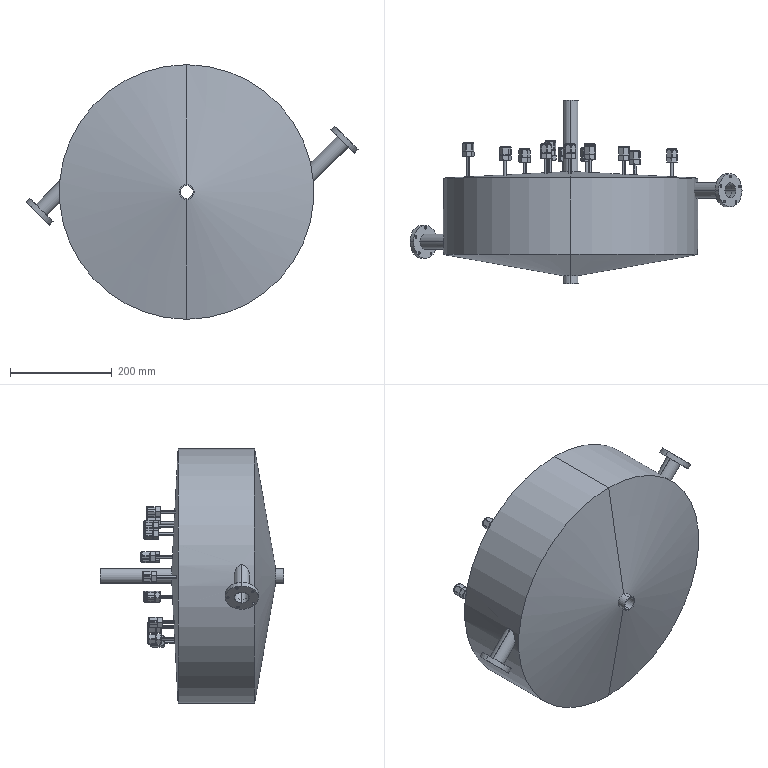Part | SolidWorks | features ReferencePattern 8, LocalLPattern 2, 3DProfileFeature 1 | 59 solids | 2913 faces | box 652.028 x 361.167 x 500 mm | volume 2508772 mm3 | cylinder 2092 | plane 362 | cone 290 | spline 169 | commonest cylinder face diameters 5 x934 15 x840 6 x108 2 x84 4 x28 16 x28